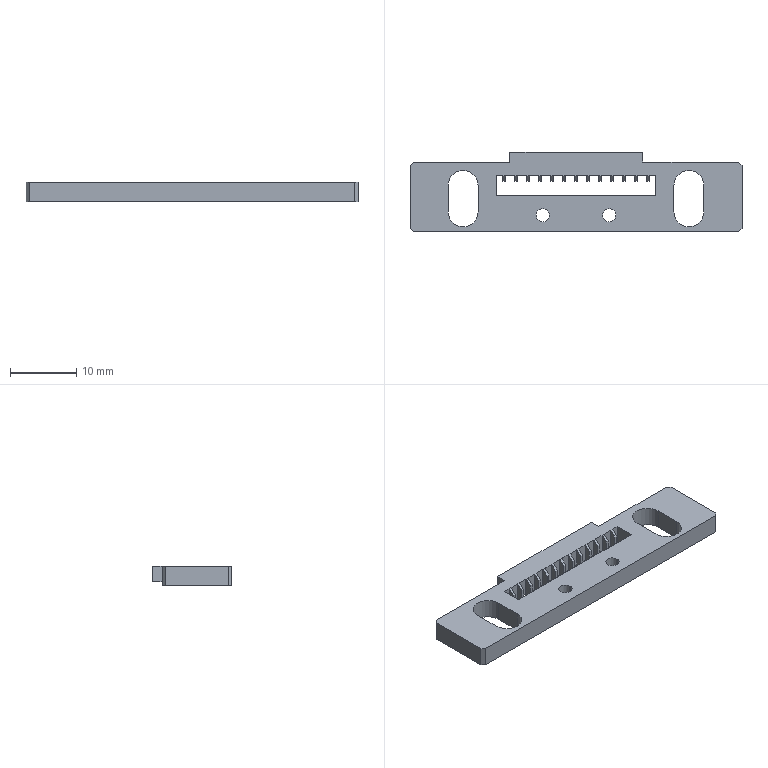Part | SolidWorks | features BaseBody 1, HoleWzd 1 | 1 solid | 122 faces | box 50 x 12 x 3 mm | volume 1210 mm3 | plane 114 | cylinder 8 | commonest cylinder face diameters 2 x4 4.5 x4